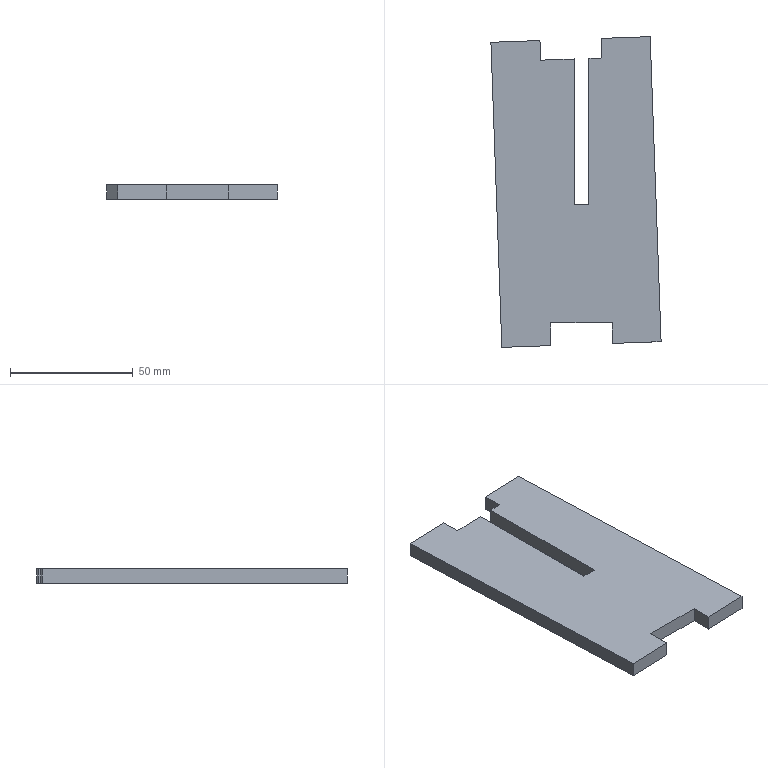Part | SolidWorks | features Extrusion 1, ICE 1 | 1 solid | 18 faces | box 69.342 x 126.628 x 6 mm | volume 43791 mm3 | plane 18
STEP:
#1=CARTESIAN_POINT('',(147.789,83.809,0.));
#2=VERTEX_POINT('',#1);
#3=CARTESIAN_POINT('',(142.514,83.62,0.));
#4=VERTEX_POINT('',#3);
#5=CARTESIAN_POINT('',(147.789,83.809,0.));
#6=DIRECTION('',(-0.9994,-0.03577,0.));
#7=VECTOR('',#6,1000.);
#8=LINE('',#5,#7);
#9=EDGE_CURVE('',#2,#4,#8,.T.);
#10=ORIENTED_EDGE('',*,*,#9,.T.);
#11=CARTESIAN_POINT('',(142.514,83.62,6.));
#12=VERTEX_POINT('',#11);
#13=CARTESIAN_POINT('',(142.514,83.62,6.));
#14=DIRECTION('',(0.,0.,1.));
#15=VECTOR('',#14,1000.);
#16=LINE('',#13,#15);
#17=EDGE_CURVE('',#4,#12,#16,.T.);
#18=ORIENTED_EDGE('',*,*,#17,.T.);
#19=CARTESIAN_POINT('',(147.789,83.809,6.));
#20=VERTEX_POINT('',#19);
#21=CARTESIAN_POINT('',(147.789,83.809,6.));
#22=DIRECTION('',(-0.9994,-0.03577,0.));
#23=VECTOR('',#22,1000.);
#24=LINE('',#21,#23);
#25=EDGE_CURVE('',#20,#12,#24,.T.);
#26=ORIENTED_EDGE('',*,*,#25,.F.);
#27=CARTESIAN_POINT('',(147.789,83.809,6.));
#28=DIRECTION('',(0.,0.,-1.));
#29=VECTOR('',#28,1000.);
#30=LINE('',#27,#29);
#31=EDGE_CURVE('',#20,#2,#30,.T.);
#32=ORIENTED_EDGE('',*,*,#31,.T.);
#33=EDGE_LOOP('',(#10,#18,#26,#32));
#34=FACE_OUTER_BOUND('',#33,.T.);
#35=CARTESIAN_POINT('',(147.789,83.809,6.));
#36=DIRECTION('',(0.03577,-0.9994,0.));
#37=DIRECTION('',(0.9994,0.03577,0.));
#38=AXIS2_PLACEMENT_3D('',#35,#36,#37);
#39=PLANE('',#38);
#40=ADVANCED_FACE('',(#34),#39,.F.);
#41=CARTESIAN_POINT('',(136.514,83.405,6.));
#42=VERTEX_POINT('',#41);
#43=CARTESIAN_POINT('',(122.85,82.916,6.));
#44=VERTEX_POINT('',#43);
#45=CARTESIAN_POINT('',(147.789,83.809,6.));
#46=DIRECTION('',(-0.9994,-0.03577,0.));
#47=VECTOR('',#46,1000.);
#48=LINE('',#45,#47);
#49=EDGE_CURVE('',#42,#44,#48,.T.);
#50=ORIENTED_EDGE('',*,*,#49,.F.);
#51=CARTESIAN_POINT('',(136.514,83.405,0.));
#52=VERTEX_POINT('',#51);
#53=CARTESIAN_POINT('',(136.514,83.405,6.));
#54=DIRECTION('',(0.,0.,-1.));
#55=VECTOR('',#54,1000.);
#56=LINE('',#53,#55);
#57=EDGE_CURVE('',#42,#52,#56,.T.);
#58=ORIENTED_EDGE('',*,*,#57,.T.);
#59=CARTESIAN_POINT('',(122.85,82.916,0.));
#60=VERTEX_POINT('',#59);
#61=CARTESIAN_POINT('',(147.789,83.809,0.));
#62=DIRECTION('',(-0.9994,-0.03577,0.));
#63=VECTOR('',#62,1000.);
#64=LINE('',#61,#63);
#65=EDGE_CURVE('',#52,#60,#64,.T.);
#66=ORIENTED_EDGE('',*,*,#65,.T.);
#67=CARTESIAN_POINT('',(122.85,82.916,6.));
#68=DIRECTION('',(0.,0.,-1.));
#69=VECTOR('',#68,1000.);
#70=LINE('',#67,#69);
#71=EDGE_CURVE('',#44,#60,#70,.T.);
#72=ORIENTED_EDGE('',*,*,#71,.F.);
#73=EDGE_LOOP('',(#50,#58,#66,#72));
#74=FACE_OUTER_BOUND('',#73,.T.);
#75=CARTESIAN_POINT('',(147.789,83.809,6.));
#76=DIRECTION('',(0.03577,-0.9994,0.));
#77=DIRECTION('',(0.9994,0.03577,0.));
#78=AXIS2_PLACEMENT_3D('',#75,#76,#77);
#79=PLANE('',#78);
#80=ADVANCED_FACE('',(#74),#79,.F.);
#81=CARTESIAN_POINT('',(122.564,90.911,0.));
#82=VERTEX_POINT('',#81);
#83=CARTESIAN_POINT('',(122.85,82.916,0.));
#84=DIRECTION('',(-0.03577,0.9994,0.));
#85=VECTOR('',#84,1000.);
#86=LINE('',#83,#85);
#87=EDGE_CURVE('',#60,#82,#86,.T.);
#88=ORIENTED_EDGE('',*,*,#87,.T.);
#89=CARTESIAN_POINT('',(122.564,90.911,6.));
#90=VERTEX_POINT('',#89);
#91=CARTESIAN_POINT('',(122.564,90.911,6.));
#92=DIRECTION('',(0.,0.,-1.));
#93=VECTOR('',#92,1000.);
#94=LINE('',#91,#93);
#95=EDGE_CURVE('',#90,#82,#94,.T.);
#96=ORIENTED_EDGE('',*,*,#95,.F.);
#97=CARTESIAN_POINT('',(122.85,82.916,6.));
#98=DIRECTION('',(-0.03577,0.9994,0.));
#99=VECTOR('',#98,1000.);
#100=LINE('',#97,#99);
#101=EDGE_CURVE('',#44,#90,#100,.T.);
#102=ORIENTED_EDGE('',*,*,#101,.F.);
#103=ORIENTED_EDGE('',*,*,#71,.T.);
#104=EDGE_LOOP('',(#88,#96,#102,#103));
#105=FACE_OUTER_BOUND('',#104,.T.);
#106=CARTESIAN_POINT('',(122.85,82.916,6.));
#107=DIRECTION('',(-0.9994,-0.03577,0.));
#108=DIRECTION('',(0.03577,-0.9994,0.));
#109=AXIS2_PLACEMENT_3D('',#106,#107,#108);
#110=PLANE('',#109);
#111=ADVANCED_FACE('',(#105),#110,.F.);
#112=CARTESIAN_POINT('',(102.587,90.196,0.));
#113=VERTEX_POINT('',#112);
#114=CARTESIAN_POINT('',(122.564,90.911,0.));
#115=DIRECTION('',(-0.9994,-0.03577,0.));
#116=VECTOR('',#115,1000.);
#117=LINE('',#114,#116);
#118=EDGE_CURVE('',#82,#113,#117,.T.);
#119=ORIENTED_EDGE('',*,*,#118,.T.);
#120=CARTESIAN_POINT('',(102.587,90.196,6.));
#121=VERTEX_POINT('',#120);
#122=CARTESIAN_POINT('',(102.587,90.196,6.));
#123=DIRECTION('',(0.,0.,-1.));
#124=VECTOR('',#123,1000.);
#125=LINE('',#122,#124);
#126=EDGE_CURVE('',#121,#113,#125,.T.);
#127=ORIENTED_EDGE('',*,*,#126,.F.);
#128=CARTESIAN_POINT('',(122.564,90.911,6.));
#129=DIRECTION('',(-0.9994,-0.03577,0.));
#130=VECTOR('',#129,1000.);
#131=LINE('',#128,#130);
#132=EDGE_CURVE('',#90,#121,#131,.T.);
#133=ORIENTED_EDGE('',*,*,#132,.F.);
#134=ORIENTED_EDGE('',*,*,#95,.T.);
#135=EDGE_LOOP('',(#119,#127,#133,#134));
#136=FACE_OUTER_BOUND('',#135,.T.);
#137=CARTESIAN_POINT('',(122.564,90.911,6.));
#138=DIRECTION('',(0.03577,-0.9994,0.));
#139=DIRECTION('',(0.9994,0.03577,0.));
#140=AXIS2_PLACEMENT_3D('',#137,#138,#139);
#141=PLANE('',#140);
#142=ADVANCED_FACE('',(#136),#141,.F.);
#143=CARTESIAN_POINT('',(107.036,-34.109,0.));
#144=VERTEX_POINT('',#143);
#145=CARTESIAN_POINT('',(107.036,-34.109,0.));
#146=DIRECTION('',(0.03577,-0.9994,0.));
#147=VECTOR('',#146,1000.);
#148=LINE('',#145,#147);
#149=EDGE_CURVE('',#113,#144,#148,.T.);
#150=ORIENTED_EDGE('',*,*,#149,.T.);
#151=CARTESIAN_POINT('',(107.036,-34.109,6.));
#152=VERTEX_POINT('',#151);
#153=CARTESIAN_POINT('',(107.036,-34.109,6.));
#154=DIRECTION('',(0.,0.,-1.));
#155=VECTOR('',#154,1000.);
#156=LINE('',#153,#155);
#157=EDGE_CURVE('',#152,#144,#156,.T.);
#158=ORIENTED_EDGE('',*,*,#157,.F.);
#159=CARTESIAN_POINT('',(107.036,-34.109,6.));
#160=DIRECTION('',(0.03577,-0.9994,0.));
#161=VECTOR('',#160,1000.);
#162=LINE('',#159,#161);
#163=EDGE_CURVE('',#121,#152,#162,.T.);
#164=ORIENTED_EDGE('',*,*,#163,.F.);
#165=ORIENTED_EDGE('',*,*,#126,.T.);
#166=EDGE_LOOP('',(#150,#158,#164,#165));
#167=FACE_OUTER_BOUND('',#166,.T.);
#168=CARTESIAN_POINT('',(107.036,-34.109,6.));
#169=DIRECTION('',(0.9994,0.03577,0.));
#170=DIRECTION('',(-0.03577,0.9994,0.));
#171=AXIS2_PLACEMENT_3D('',#168,#169,#170);
#172=PLANE('',#171);
#173=ADVANCED_FACE('',(#167),#172,.F.);
#174=CARTESIAN_POINT('',(127.013,-33.394,0.));
#175=VERTEX_POINT('',#174);
#176=CARTESIAN_POINT('',(107.036,-34.109,0.));
#177=DIRECTION('',(0.9994,0.03577,0.));
#178=VECTOR('',#177,1000.);
#179=LINE('',#176,#178);
#180=EDGE_CURVE('',#144,#175,#179,.T.);
#181=ORIENTED_EDGE('',*,*,#180,.T.);
#182=CARTESIAN_POINT('',(127.013,-33.394,6.));
#183=VERTEX_POINT('',#182);
#184=CARTESIAN_POINT('',(127.013,-33.394,6.));
#185=DIRECTION('',(0.,0.,-1.));
#186=VECTOR('',#185,1000.);
#187=LINE('',#184,#186);
#188=EDGE_CURVE('',#183,#175,#187,.T.);
#189=ORIENTED_EDGE('',*,*,#188,.F.);
#190=CARTESIAN_POINT('',(107.036,-34.109,6.));
#191=DIRECTION('',(0.9994,0.03577,0.));
#192=VECTOR('',#191,1000.);
#193=LINE('',#190,#192);
#194=EDGE_CURVE('',#152,#183,#193,.T.);
#195=ORIENTED_EDGE('',*,*,#194,.F.);
#196=ORIENTED_EDGE('',*,*,#157,.T.);
#197=EDGE_LOOP('',(#181,#189,#195,#196));
#198=FACE_OUTER_BOUND('',#197,.T.);
#199=CARTESIAN_POINT('',(107.036,-34.109,6.));
#200=DIRECTION('',(-0.03577,0.9994,0.));
#201=DIRECTION('',(-0.9994,-0.03577,0.));
#202=AXIS2_PLACEMENT_3D('',#199,#200,#201);
#203=PLANE('',#202);
#204=ADVANCED_FACE('',(#198),#203,.F.);
#205=CARTESIAN_POINT('',(127.013,-24.109,0.));
#206=VERTEX_POINT('',#205);
#207=CARTESIAN_POINT('',(127.013,-33.394,0.));
#208=DIRECTION('',(0.,1.,0.));
#209=VECTOR('',#208,1000.);
#210=LINE('',#207,#209);
#211=EDGE_CURVE('',#175,#206,#210,.T.);
#212=ORIENTED_EDGE('',*,*,#211,.T.);
#213=CARTESIAN_POINT('',(127.013,-24.109,6.));
#214=VERTEX_POINT('',#213);
#215=CARTESIAN_POINT('',(127.013,-24.109,6.));
#216=DIRECTION('',(0.,0.,-1.));
#217=VECTOR('',#216,1000.);
#218=LINE('',#215,#217);
#219=EDGE_CURVE('',#214,#206,#218,.T.);
#220=ORIENTED_EDGE('',*,*,#219,.F.);
#221=CARTESIAN_POINT('',(127.013,-33.394,6.));
#222=DIRECTION('',(0.,1.,0.));
#223=VECTOR('',#222,1000.);
#224=LINE('',#221,#223);
#225=EDGE_CURVE('',#183,#214,#224,.T.);
#226=ORIENTED_EDGE('',*,*,#225,.F.);
#227=ORIENTED_EDGE('',*,*,#188,.T.);
#228=EDGE_LOOP('',(#212,#220,#226,#227));
#229=FACE_OUTER_BOUND('',#228,.T.);
#230=CARTESIAN_POINT('',(127.013,-33.394,6.));
#231=DIRECTION('',(-1.,0.,0.));
#232=DIRECTION('',(0.,0.,1.));
#233=AXIS2_PLACEMENT_3D('',#230,#231,#232);
#234=PLANE('',#233);
#235=ADVANCED_FACE('',(#229),#234,.F.);
#236=CARTESIAN_POINT('',(152.014,-24.109,0.));
#237=VERTEX_POINT('',#236);
#238=CARTESIAN_POINT('',(127.013,-24.109,0.));
#239=DIRECTION('',(1.,0.,0.));
#240=VECTOR('',#239,1000.);
#241=LINE('',#238,#240);
#242=EDGE_CURVE('',#206,#237,#241,.T.);
#243=ORIENTED_EDGE('',*,*,#242,.T.);
#244=CARTESIAN_POINT('',(152.014,-24.109,6.));
#245=VERTEX_POINT('',#244);
#246=CARTESIAN_POINT('',(152.014,-24.109,6.));
#247=DIRECTION('',(0.,0.,-1.));
#248=VECTOR('',#247,1000.);
#249=LINE('',#246,#248);
#250=EDGE_CURVE('',#245,#237,#249,.T.);
#251=ORIENTED_EDGE('',*,*,#250,.F.);
#252=CARTESIAN_POINT('',(127.013,-24.109,6.));
#253=DIRECTION('',(1.,0.,0.));
#254=VECTOR('',#253,1000.);
#255=LINE('',#252,#254);
#256=EDGE_CURVE('',#214,#245,#255,.T.);
#257=ORIENTED_EDGE('',*,*,#256,.F.);
#258=ORIENTED_EDGE('',*,*,#219,.T.);
#259=EDGE_LOOP('',(#243,#251,#257,#258));
#260=FACE_OUTER_BOUND('',#259,.T.);
#261=CARTESIAN_POINT('',(127.013,-24.109,6.));
#262=DIRECTION('',(0.,1.,0.));
#263=DIRECTION('',(0.,0.,1.));
#264=AXIS2_PLACEMENT_3D('',#261,#262,#263);
#265=PLANE('',#264);
#266=ADVANCED_FACE('',(#260),#265,.F.);
#267=CARTESIAN_POINT('',(152.014,-32.499,0.));
#268=VERTEX_POINT('',#267);
#269=CARTESIAN_POINT('',(152.014,-24.109,0.));
#270=DIRECTION('',(0.,-1.,0.));
#271=VECTOR('',#270,1000.);
#272=LINE('',#269,#271);
#273=EDGE_CURVE('',#237,#268,#272,.T.);
#274=ORIENTED_EDGE('',*,*,#273,.T.);
#275=CARTESIAN_POINT('',(152.014,-32.499,6.));
#276=VERTEX_POINT('',#275);
#277=CARTESIAN_POINT('',(152.014,-32.499,6.));
#278=DIRECTION('',(0.,0.,-1.));
#279=VECTOR('',#278,1000.);
#280=LINE('',#277,#279);
#281=EDGE_CURVE('',#276,#268,#280,.T.);
#282=ORIENTED_EDGE('',*,*,#281,.F.);
#283=CARTESIAN_POINT('',(152.014,-24.109,6.));
#284=DIRECTION('',(0.,-1.,0.));
#285=VECTOR('',#284,1000.);
#286=LINE('',#283,#285);
#287=EDGE_CURVE('',#245,#276,#286,.T.);
#288=ORIENTED_EDGE('',*,*,#287,.F.);
#289=ORIENTED_EDGE('',*,*,#250,.T.);
#290=EDGE_LOOP('',(#274,#282,#288,#289));
#291=FACE_OUTER_BOUND('',#290,.T.);
#292=CARTESIAN_POINT('',(152.014,-24.109,6.));
#293=DIRECTION('',(1.,0.,0.));
#294=DIRECTION('',(0.,0.,-1.));
#295=AXIS2_PLACEMENT_3D('',#292,#293,#294);
#296=PLANE('',#295);
#297=ADVANCED_FACE('',(#291),#296,.F.);
#298=CARTESIAN_POINT('',(171.929,-31.786,0.));
#299=VERTEX_POINT('',#298);
#300=CARTESIAN_POINT('',(152.014,-32.499,0.));
#301=DIRECTION('',(0.9994,0.03577,0.));
#302=VECTOR('',#301,1000.);
#303=LINE('',#300,#302);
#304=EDGE_CURVE('',#268,#299,#303,.T.);
#305=ORIENTED_EDGE('',*,*,#304,.T.);
#306=CARTESIAN_POINT('',(171.929,-31.786,6.));
#307=VERTEX_POINT('',#306);
#308=CARTESIAN_POINT('',(171.929,-31.786,6.));
#309=DIRECTION('',(0.,0.,-1.));
#310=VECTOR('',#309,1000.);
#311=LINE('',#308,#310);
#312=EDGE_CURVE('',#307,#299,#311,.T.);
#313=ORIENTED_EDGE('',*,*,#312,.F.);
#314=CARTESIAN_POINT('',(152.014,-32.499,6.));
#315=DIRECTION('',(0.9994,0.03577,0.));
#316=VECTOR('',#315,1000.);
#317=LINE('',#314,#316);
#318=EDGE_CURVE('',#276,#307,#317,.T.);
#319=ORIENTED_EDGE('',*,*,#318,.F.);
#320=ORIENTED_EDGE('',*,*,#281,.T.);
#321=EDGE_LOOP('',(#305,#313,#319,#320));
#322=FACE_OUTER_BOUND('',#321,.T.);
#323=CARTESIAN_POINT('',(152.014,-32.499,6.));
#324=DIRECTION('',(-0.03577,0.9994,0.));
#325=DIRECTION('',(-0.9994,-0.03577,0.));
#326=AXIS2_PLACEMENT_3D('',#323,#324,#325);
#327=PLANE('',#326);
#328=ADVANCED_FACE('',(#322),#327,.F.);
#329=CARTESIAN_POINT('',(167.479,92.519,0.));
#330=VERTEX_POINT('',#329);
#331=CARTESIAN_POINT('',(171.929,-31.786,0.));
#332=DIRECTION('',(-0.03577,0.9994,0.));
#333=VECTOR('',#332,1000.);
#334=LINE('',#331,#333);
#335=EDGE_CURVE('',#299,#330,#334,.T.);
#336=ORIENTED_EDGE('',*,*,#335,.T.);
#337=CARTESIAN_POINT('',(167.479,92.519,6.));
#338=VERTEX_POINT('',#337);
#339=CARTESIAN_POINT('',(167.479,92.519,6.));
#340=DIRECTION('',(0.,0.,-1.));
#341=VECTOR('',#340,1000.);
#342=LINE('',#339,#341);
#343=EDGE_CURVE('',#338,#330,#342,.T.);
#344=ORIENTED_EDGE('',*,*,#343,.F.);
#345=CARTESIAN_POINT('',(171.929,-31.786,6.));
#346=DIRECTION('',(-0.03577,0.9994,0.));
#347=VECTOR('',#346,1000.);
#348=LINE('',#345,#347);
#349=EDGE_CURVE('',#307,#338,#348,.T.);
#350=ORIENTED_EDGE('',*,*,#349,.F.);
#351=ORIENTED_EDGE('',*,*,#312,.T.);
#352=EDGE_LOOP('',(#336,#344,#350,#351));
#353=FACE_OUTER_BOUND('',#352,.T.);
#354=CARTESIAN_POINT('',(171.929,-31.786,6.));
#355=DIRECTION('',(-0.9994,-0.03577,0.));
#356=DIRECTION('',(0.03577,-0.9994,0.));
#357=AXIS2_PLACEMENT_3D('',#354,#355,#356);
#358=PLANE('',#357);
#359=ADVANCED_FACE('',(#353),#358,.F.);
#360=CARTESIAN_POINT('',(147.503,91.804,0.));
#361=VERTEX_POINT('',#360);
#362=CARTESIAN_POINT('',(147.503,91.804,0.));
#363=DIRECTION('',(-0.9994,-0.03577,0.));
#364=VECTOR('',#363,1000.);
#365=LINE('',#362,#364);
#366=EDGE_CURVE('',#330,#361,#365,.T.);
#367=ORIENTED_EDGE('',*,*,#366,.T.);
#368=CARTESIAN_POINT('',(147.503,91.804,6.));
#369=VERTEX_POINT('',#368);
#370=CARTESIAN_POINT('',(147.503,91.804,6.));
#371=DIRECTION('',(0.,0.,-1.));
#372=VECTOR('',#371,1000.);
#373=LINE('',#370,#372);
#374=EDGE_CURVE('',#369,#361,#373,.T.);
#375=ORIENTED_EDGE('',*,*,#374,.F.);
#376=CARTESIAN_POINT('',(147.503,91.804,6.));
#377=DIRECTION('',(-0.9994,-0.03577,0.));
#378=VECTOR('',#377,1000.);
#379=LINE('',#376,#378);
#380=EDGE_CURVE('',#338,#369,#379,.T.);
#381=ORIENTED_EDGE('',*,*,#380,.F.);
#382=ORIENTED_EDGE('',*,*,#343,.T.);
#383=EDGE_LOOP('',(#367,#375,#381,#382));
#384=FACE_OUTER_BOUND('',#383,.T.);
#385=CARTESIAN_POINT('',(147.503,91.804,6.));
#386=DIRECTION('',(0.03577,-0.9994,0.));
#387=DIRECTION('',(0.9994,0.03577,0.));
#388=AXIS2_PLACEMENT_3D('',#385,#386,#387);
#389=PLANE('',#388);
#390=ADVANCED_FACE('',(#384),#389,.F.);
#391=CARTESIAN_POINT('',(147.789,83.809,0.));
#392=DIRECTION('',(0.03577,-0.9994,0.));
#393=VECTOR('',#392,1000.);
#394=LINE('',#391,#393);
#395=EDGE_CURVE('',#361,#2,#394,.T.);
#396=ORIENTED_EDGE('',*,*,#395,.T.);
#397=ORIENTED_EDGE('',*,*,#31,.F.);
#398=CARTESIAN_POINT('',(147.789,83.809,6.));
#399=DIRECTION('',(0.03577,-0.9994,0.));
#400=VECTOR('',#399,1000.);
#401=LINE('',#398,#400);
#402=EDGE_CURVE('',#369,#20,#401,.T.);
#403=ORIENTED_EDGE('',*,*,#402,.F.);
#404=ORIENTED_EDGE('',*,*,#374,.T.);
#405=EDGE_LOOP('',(#396,#397,#403,#404));
#406=FACE_OUTER_BOUND('',#405,.T.);
#407=CARTESIAN_POINT('',(147.789,83.809,6.));
#408=DIRECTION('',(0.9994,0.03577,0.));
#409=DIRECTION('',(-0.03577,0.9994,0.));
#410=AXIS2_PLACEMENT_3D('',#407,#408,#409);
#411=PLANE('',#410);
#412=ADVANCED_FACE('',(#406),#411,.F.);
#413=ORIENTED_EDGE('',*,*,#25,.T.);
#414=CARTESIAN_POINT('',(142.514,23.91,6.));
#415=VERTEX_POINT('',#414);
#416=CARTESIAN_POINT('',(142.514,83.886,6.));
#417=DIRECTION('',(0.,1.,0.));
#418=VECTOR('',#417,1000.);
#419=LINE('',#416,#418);
#420=EDGE_CURVE('',#415,#12,#419,.T.);
#421=ORIENTED_EDGE('',*,*,#420,.F.);
#422=CARTESIAN_POINT('',(136.514,23.91,6.));
#423=VERTEX_POINT('',#422);
#424=CARTESIAN_POINT('',(136.514,23.91,6.));
#425=DIRECTION('',(1.,0.,0.));
#426=VECTOR('',#425,1000.);
#427=LINE('',#424,#426);
#428=EDGE_CURVE('',#423,#415,#427,.T.);
#429=ORIENTED_EDGE('',*,*,#428,.F.);
#430=CARTESIAN_POINT('',(136.514,83.886,6.));
#431=DIRECTION('',(0.,-1.,0.));
#432=VECTOR('',#431,1000.);
#433=LINE('',#430,#432);
#434=EDGE_CURVE('',#42,#423,#433,.T.);
#435=ORIENTED_EDGE('',*,*,#434,.F.);
#436=ORIENTED_EDGE('',*,*,#49,.T.);
#437=ORIENTED_EDGE('',*,*,#101,.T.);
#438=ORIENTED_EDGE('',*,*,#132,.T.);
#439=ORIENTED_EDGE('',*,*,#163,.T.);
#440=ORIENTED_EDGE('',*,*,#194,.T.);
#441=ORIENTED_EDGE('',*,*,#225,.T.);
#442=ORIENTED_EDGE('',*,*,#256,.T.);
#443=ORIENTED_EDGE('',*,*,#287,.T.);
#444=ORIENTED_EDGE('',*,*,#318,.T.);
#445=ORIENTED_EDGE('',*,*,#349,.T.);
#446=ORIENTED_EDGE('',*,*,#380,.T.);
#447=ORIENTED_EDGE('',*,*,#402,.T.);
#448=EDGE_LOOP('',(#413,#421,#429,#435,#436,#437,#438,#439,#440,#441,#442,#443,#444,#445,#446,#447));
#449=FACE_OUTER_BOUND('',#448,.T.);
#450=CARTESIAN_POINT('',(0.,0.,6.));
#451=DIRECTION('',(0.,0.,-1.));
#452=DIRECTION('',(-1.,0.,0.));
#453=AXIS2_PLACEMENT_3D('',#450,#451,#452);
#454=PLANE('',#453);
#455=ADVANCED_FACE('',(#449),#454,.F.);
#456=CARTESIAN_POINT('',(142.514,23.91,0.));
#457=VERTEX_POINT('',#456);
#458=CARTESIAN_POINT('',(142.514,83.886,0.));
#459=DIRECTION('',(0.,1.,0.));
#460=VECTOR('',#459,1000.);
#461=LINE('',#458,#460);
#462=EDGE_CURVE('',#457,#4,#461,.T.);
#463=ORIENTED_EDGE('',*,*,#462,.T.);
#464=ORIENTED_EDGE('',*,*,#9,.F.);
#465=ORIENTED_EDGE('',*,*,#395,.F.);
#466=ORIENTED_EDGE('',*,*,#366,.F.);
#467=ORIENTED_EDGE('',*,*,#335,.F.);
#468=ORIENTED_EDGE('',*,*,#304,.F.);
#469=ORIENTED_EDGE('',*,*,#273,.F.);
#470=ORIENTED_EDGE('',*,*,#242,.F.);
#471=ORIENTED_EDGE('',*,*,#211,.F.);
#472=ORIENTED_EDGE('',*,*,#180,.F.);
#473=ORIENTED_EDGE('',*,*,#149,.F.);
#474=ORIENTED_EDGE('',*,*,#118,.F.);
#475=ORIENTED_EDGE('',*,*,#87,.F.);
#476=ORIENTED_EDGE('',*,*,#65,.F.);
#477=CARTESIAN_POINT('',(136.514,23.91,0.));
#478=VERTEX_POINT('',#477);
#479=CARTESIAN_POINT('',(136.514,0.,0.));
#480=DIRECTION('',(0.,1.,0.));
#481=VECTOR('',#480,1000.);
#482=LINE('',#479,#481);
#483=EDGE_CURVE('',#478,#52,#482,.T.);
#484=ORIENTED_EDGE('',*,*,#483,.F.);
#485=CARTESIAN_POINT('',(136.514,23.91,0.));
#486=DIRECTION('',(1.,0.,0.));
#487=VECTOR('',#486,1000.);
#488=LINE('',#485,#487);
#489=EDGE_CURVE('',#478,#457,#488,.T.);
#490=ORIENTED_EDGE('',*,*,#489,.T.);
#491=EDGE_LOOP('',(#463,#464,#465,#466,#467,#468,#469,#470,#471,#472,#473,#474,#475,#476,#484,#490));
#492=FACE_OUTER_BOUND('',#491,.T.);
#493=CARTESIAN_POINT('',(0.,0.,0.));
#494=DIRECTION('',(0.,0.,-1.));
#495=DIRECTION('',(-1.,0.,0.));
#496=AXIS2_PLACEMENT_3D('',#493,#494,#495);
#497=PLANE('',#496);
#498=ADVANCED_FACE('',(#492),#497,.T.);
#499=ORIENTED_EDGE('',*,*,#462,.F.);
#500=CARTESIAN_POINT('',(142.514,23.91,0.));
#501=DIRECTION('',(0.,0.,1.));
#502=VECTOR('',#501,1000.);
#503=LINE('',#500,#502);
#504=EDGE_CURVE('',#457,#415,#503,.T.);
#505=ORIENTED_EDGE('',*,*,#504,.T.);
#506=ORIENTED_EDGE('',*,*,#420,.T.);
#507=ORIENTED_EDGE('',*,*,#17,.F.);
#508=EDGE_LOOP('',(#499,#505,#506,#507));
#509=FACE_OUTER_BOUND('',#508,.T.);
#510=CARTESIAN_POINT('',(142.514,83.886,0.));
#511=DIRECTION('',(1.,0.,0.));
#512=DIRECTION('',(0.,0.,-1.));
#513=AXIS2_PLACEMENT_3D('',#510,#511,#512);
#514=PLANE('',#513);
#515=ADVANCED_FACE('',(#509),#514,.F.);
#516=ORIENTED_EDGE('',*,*,#434,.T.);
#517=CARTESIAN_POINT('',(136.514,23.91,0.));
#518=DIRECTION('',(0.,0.,1.));
#519=VECTOR('',#518,1000.);
#520=LINE('',#517,#519);
#521=EDGE_CURVE('',#478,#423,#520,.T.);
#522=ORIENTED_EDGE('',*,*,#521,.F.);
#523=ORIENTED_EDGE('',*,*,#483,.T.);
#524=ORIENTED_EDGE('',*,*,#57,.F.);
#525=EDGE_LOOP('',(#516,#522,#523,#524));
#526=FACE_OUTER_BOUND('',#525,.T.);
#527=CARTESIAN_POINT('',(136.514,83.886,0.));
#528=DIRECTION('',(-1.,0.,0.));
#529=DIRECTION('',(0.,0.,1.));
#530=AXIS2_PLACEMENT_3D('',#527,#528,#529);
#531=PLANE('',#530);
#532=ADVANCED_FACE('',(#526),#531,.F.);
#533=ORIENTED_EDGE('',*,*,#428,.T.);
#534=ORIENTED_EDGE('',*,*,#504,.F.);
#535=ORIENTED_EDGE('',*,*,#489,.F.);
#536=ORIENTED_EDGE('',*,*,#521,.T.);
#537=EDGE_LOOP('',(#533,#534,#535,#536));
#538=FACE_OUTER_BOUND('',#537,.T.);
#539=CARTESIAN_POINT('',(136.514,23.91,0.));
#540=DIRECTION('',(0.,-1.,0.));
#541=DIRECTION('',(0.,0.,-1.));
#542=AXIS2_PLACEMENT_3D('',#539,#540,#541);
#543=PLANE('',#542);
#544=ADVANCED_FACE('',(#538),#543,.F.);
#545=CLOSED_SHELL('',(#40,#80,#111,#142,#173,#204,#235,#266,#297,#328,#359,#390,#412,#455,#498,#515,#532,#544));
#546=MANIFOLD_SOLID_BREP('',#545);
#547=CARTESIAN_POINT('',(0.,0.,0.));
#548=DIRECTION('',(0.,0.,1.));
#549=DIRECTION('',(1.,0.,0.));
#550=AXIS2_PLACEMENT_3D('',#547,#548,#549);
#551=(LENGTH_UNIT()NAMED_UNIT(*)SI_UNIT(.MILLI.,.METRE.));
#552=UNCERTAINTY_MEASURE_WITH_UNIT(LENGTH_MEASURE(0.00001),#551,'','');
#553=(NAMED_UNIT(*)PLANE_ANGLE_UNIT()SI_UNIT($,.RADIAN.));
#554=(NAMED_UNIT(*)SI_UNIT($,.STERADIAN.)SOLID_ANGLE_UNIT());
#555=(GEOMETRIC_REPRESENTATION_CONTEXT(3)GLOBAL_UNCERTAINTY_ASSIGNED_CONTEXT((#552))GLOBAL_UNIT_ASSIGNED_CONTEXT((#551,#553,#554))REPRESENTATION_CONTEXT('',''));
#556=ADVANCED_BREP_SHAPE_REPRESENTATION('',(#546,#550),#555);